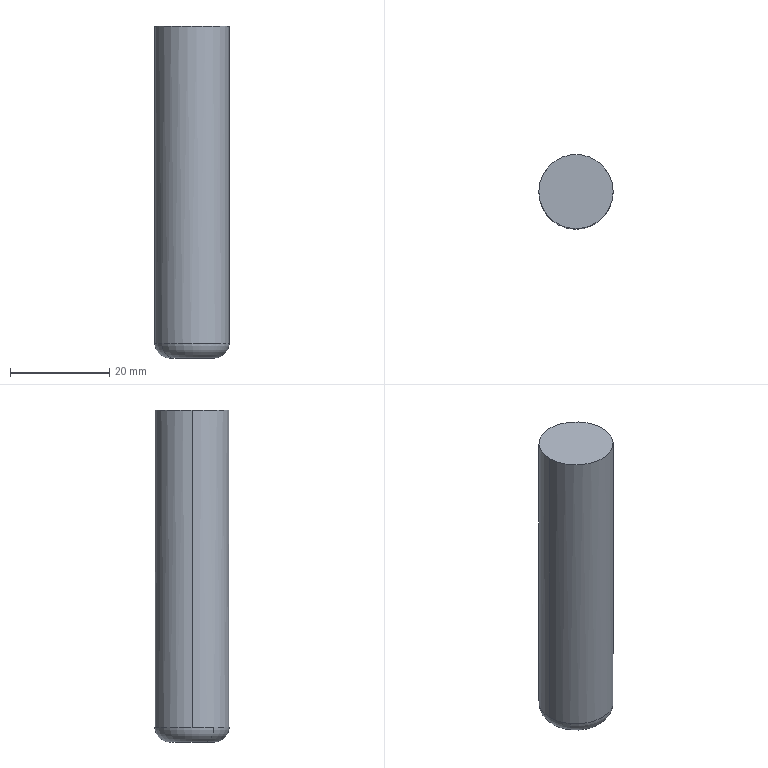Part | 1 solid | 6 faces | box 15 x 15 x 67 mm | volume 11757 mm3 | cylinder 2 | torus 2 | plane 2 | commonest cylinder face diameters 15 x2
STEP:
#1=CARTESIAN_POINT('',(0.,0.,0.));
#2=DIRECTION('',(0.,0.,1.));
#3=DIRECTION('',(1.,0.,0.));
#4=AXIS2_PLACEMENT_3D('',#1,#2,#3);
#5=CARTESIAN_POINT('',(-168.248,494.5,-238.55));
#6=VERTEX_POINT('',#5);
#7=CARTESIAN_POINT('',(-168.248,494.5,-302.55));
#8=VERTEX_POINT('',#7);
#9=CARTESIAN_POINT('',(-168.248,494.5,-238.55));
#10=DIRECTION('',(0.,0.,-1.));
#11=VECTOR('',#10,1.);
#12=LINE('',#9,#11);
#13=CARTESIAN_POINT('',(-160.748,494.5,-238.55));
#14=DIRECTION('',(0.,0.,-1.));
#15=DIRECTION('',(0.,-1.,0.));
#16=AXIS2_PLACEMENT_3D('',#13,#14,#15);
#17=CYLINDRICAL_SURFACE('',#16,7.5);
#18=CARTESIAN_POINT('',(1.571,0.));
#19=DIRECTION('',(0.,1.));
#20=VECTOR('',#19,1.);
#21=LINE('',#18,#20);
#22=(GEOMETRIC_REPRESENTATION_CONTEXT(2)PARAMETRIC_REPRESENTATION_CONTEXT()REPRESENTATION_CONTEXT('',''));
#23=DEFINITIONAL_REPRESENTATION('',(#21),#22);
#24=PCURVE('',#17,#23);
#25=CARTESIAN_POINT('',(-160.748,494.5,-238.55));
#26=DIRECTION('',(0.,0.,-1.));
#27=DIRECTION('',(0.,1.,0.));
#28=AXIS2_PLACEMENT_3D('',#25,#26,#27);
#29=CYLINDRICAL_SURFACE('',#28,7.5);
#30=CARTESIAN_POINT('',(4.712,0.));
#31=DIRECTION('',(0.,1.));
#32=VECTOR('',#31,1.);
#33=LINE('',#30,#32);
#34=(GEOMETRIC_REPRESENTATION_CONTEXT(2)PARAMETRIC_REPRESENTATION_CONTEXT()REPRESENTATION_CONTEXT('',''));
#35=DEFINITIONAL_REPRESENTATION('',(#33),#34);
#36=PCURVE('',#29,#35);
#37=SURFACE_CURVE('',#12,(#24,#36),.PCURVE_S1.);
#38=EDGE_CURVE('',#6,#8,#37,.T.);
#39=ORIENTED_EDGE('',*,*,#38,.F.);
#40=CARTESIAN_POINT('',(-153.248,494.5,-238.55));
#41=VERTEX_POINT('',#40);
#42=CARTESIAN_POINT('',(-160.748,494.5,-238.55));
#43=DIRECTION('',(0.,0.,-1.));
#44=DIRECTION('',(1.,0.,0.));
#45=AXIS2_PLACEMENT_3D('',#42,#43,#44);
#46=CIRCLE('',#45,7.5);
#47=CARTESIAN_POINT('',(-1.571,0.));
#48=DIRECTION('',(1.,0.));
#49=VECTOR('',#48,1.);
#50=LINE('',#47,#49);
#51=(GEOMETRIC_REPRESENTATION_CONTEXT(2)PARAMETRIC_REPRESENTATION_CONTEXT()REPRESENTATION_CONTEXT('',''));
#52=DEFINITIONAL_REPRESENTATION('',(#50),#51);
#53=PCURVE('',#17,#52);
#54=CARTESIAN_POINT('',(-160.748,494.5,-238.55));
#55=DIRECTION('',(0.,0.,-1.));
#56=DIRECTION('',(1.,0.,0.));
#57=AXIS2_PLACEMENT_3D('',#54,#55,#56);
#58=PLANE('',#57);
#59=CARTESIAN_POINT('',(0.,0.));
#60=DIRECTION('',(1.,0.));
#61=AXIS2_PLACEMENT_2D('',#59,#60);
#62=CIRCLE('',#61,7.5);
#63=(GEOMETRIC_REPRESENTATION_CONTEXT(2)PARAMETRIC_REPRESENTATION_CONTEXT()REPRESENTATION_CONTEXT('',''));
#64=DEFINITIONAL_REPRESENTATION('',(#62),#63);
#65=PCURVE('',#58,#64);
#66=SURFACE_CURVE('',#46,(#53,#65),.PCURVE_S1.);
#67=EDGE_CURVE('',#6,#41,#66,.T.);
#68=ORIENTED_EDGE('',*,*,#67,.T.);
#69=CARTESIAN_POINT('',(-153.248,494.5,-302.55));
#70=VERTEX_POINT('',#69);
#71=CARTESIAN_POINT('',(-153.248,494.5,-238.55));
#72=DIRECTION('',(0.,0.,-1.));
#73=VECTOR('',#72,1.);
#74=LINE('',#71,#73);
#75=CARTESIAN_POINT('',(4.712,0.));
#76=DIRECTION('',(0.,1.));
#77=VECTOR('',#76,1.);
#78=LINE('',#75,#77);
#79=(GEOMETRIC_REPRESENTATION_CONTEXT(2)PARAMETRIC_REPRESENTATION_CONTEXT()REPRESENTATION_CONTEXT('',''));
#80=DEFINITIONAL_REPRESENTATION('',(#78),#79);
#81=PCURVE('',#17,#80);
#82=CARTESIAN_POINT('',(1.571,0.));
#83=DIRECTION('',(0.,1.));
#84=VECTOR('',#83,1.);
#85=LINE('',#82,#84);
#86=(GEOMETRIC_REPRESENTATION_CONTEXT(2)PARAMETRIC_REPRESENTATION_CONTEXT()REPRESENTATION_CONTEXT('',''));
#87=DEFINITIONAL_REPRESENTATION('',(#85),#86);
#88=PCURVE('',#29,#87);
#89=SURFACE_CURVE('',#74,(#81,#88),.PCURVE_S1.);
#90=EDGE_CURVE('',#41,#70,#89,.T.);
#91=ORIENTED_EDGE('',*,*,#90,.T.);
#92=CARTESIAN_POINT('',(-154.68,498.909,-302.55));
#93=VERTEX_POINT('',#92);
#94=CARTESIAN_POINT('',(-160.748,494.5,-302.55));
#95=DIRECTION('',(0.,0.,1.));
#96=DIRECTION('',(-0.809,0.5878,0.));
#97=AXIS2_PLACEMENT_3D('',#94,#95,#96);
#98=CIRCLE('',#97,7.5);
#99=CARTESIAN_POINT('',(8.482,64.));
#100=DIRECTION('',(-1.,0.));
#101=VECTOR('',#100,1.);
#102=LINE('',#99,#101);
#103=(GEOMETRIC_REPRESENTATION_CONTEXT(2)PARAMETRIC_REPRESENTATION_CONTEXT()REPRESENTATION_CONTEXT('',''));
#104=DEFINITIONAL_REPRESENTATION('',(#102),#103);
#105=PCURVE('',#17,#104);
#106=CARTESIAN_POINT('',(-160.748,494.5,-302.55));
#107=DIRECTION('',(0.,0.,-1.));
#108=DIRECTION('',(-0.5878,0.809,0.));
#109=AXIS2_PLACEMENT_3D('',#106,#107,#108);
#110=TOROIDAL_SURFACE('',#109,4.5,3.);
#111=CARTESIAN_POINT('',(5.969,0.));
#112=DIRECTION('',(-1.,0.));
#113=VECTOR('',#112,1.);
#114=LINE('',#111,#113);
#115=(GEOMETRIC_REPRESENTATION_CONTEXT(2)PARAMETRIC_REPRESENTATION_CONTEXT()REPRESENTATION_CONTEXT('',''));
#116=DEFINITIONAL_REPRESENTATION('',(#114),#115);
#117=PCURVE('',#110,#116);
#118=SURFACE_CURVE('',#98,(#105,#117),.PCURVE_S1.);
#119=EDGE_CURVE('',#70,#93,#118,.T.);
#120=ORIENTED_EDGE('',*,*,#119,.T.);
#121=CARTESIAN_POINT('',(-166.815,498.909,-302.55));
#122=VERTEX_POINT('',#121);
#123=CARTESIAN_POINT('',(-160.748,494.5,-302.55));
#124=DIRECTION('',(0.,0.,1.));
#125=DIRECTION('',(-0.809,0.5878,0.));
#126=AXIS2_PLACEMENT_3D('',#123,#124,#125);
#127=CIRCLE('',#126,7.5);
#128=CARTESIAN_POINT('',(8.482,64.));
#129=DIRECTION('',(-1.,0.));
#130=VECTOR('',#129,1.);
#131=LINE('',#128,#130);
#132=(GEOMETRIC_REPRESENTATION_CONTEXT(2)PARAMETRIC_REPRESENTATION_CONTEXT()REPRESENTATION_CONTEXT('',''));
#133=DEFINITIONAL_REPRESENTATION('',(#131),#132);
#134=PCURVE('',#17,#133);
#135=CARTESIAN_POINT('',(-160.748,494.5,-302.55));
#136=DIRECTION('',(0.,0.,-1.));
#137=DIRECTION('',(0.5878,-0.809,0.));
#138=AXIS2_PLACEMENT_3D('',#135,#136,#137);
#139=TOROIDAL_SURFACE('',#138,4.5,3.);
#140=CARTESIAN_POINT('',(9.111,0.));
#141=DIRECTION('',(-1.,0.));
#142=VECTOR('',#141,1.);
#143=LINE('',#140,#142);
#144=(GEOMETRIC_REPRESENTATION_CONTEXT(2)PARAMETRIC_REPRESENTATION_CONTEXT()REPRESENTATION_CONTEXT('',''));
#145=DEFINITIONAL_REPRESENTATION('',(#143),#144);
#146=PCURVE('',#139,#145);
#147=SURFACE_CURVE('',#127,(#134,#146),.PCURVE_S1.);
#148=EDGE_CURVE('',#93,#122,#147,.T.);
#149=ORIENTED_EDGE('',*,*,#148,.T.);
#150=CARTESIAN_POINT('',(-160.748,494.5,-302.55));
#151=DIRECTION('',(0.,0.,1.));
#152=DIRECTION('',(-0.809,0.5878,0.));
#153=AXIS2_PLACEMENT_3D('',#150,#151,#152);
#154=CIRCLE('',#153,7.5);
#155=CARTESIAN_POINT('',(2.199,64.));
#156=DIRECTION('',(-1.,0.));
#157=VECTOR('',#156,1.);
#158=LINE('',#155,#157);
#159=(GEOMETRIC_REPRESENTATION_CONTEXT(2)PARAMETRIC_REPRESENTATION_CONTEXT()REPRESENTATION_CONTEXT('',''));
#160=DEFINITIONAL_REPRESENTATION('',(#158),#159);
#161=PCURVE('',#17,#160);
#162=CARTESIAN_POINT('',(2.827,0.));
#163=DIRECTION('',(-1.,0.));
#164=VECTOR('',#163,1.);
#165=LINE('',#162,#164);
#166=(GEOMETRIC_REPRESENTATION_CONTEXT(2)PARAMETRIC_REPRESENTATION_CONTEXT()REPRESENTATION_CONTEXT('',''));
#167=DEFINITIONAL_REPRESENTATION('',(#165),#166);
#168=PCURVE('',#139,#167);
#169=SURFACE_CURVE('',#154,(#161,#168),.PCURVE_S1.);
#170=EDGE_CURVE('',#122,#8,#169,.T.);
#171=ORIENTED_EDGE('',*,*,#170,.T.);
#172=EDGE_LOOP('',(#39,#68,#91,#120,#149,#171));
#173=FACE_BOUND('',#172,.T.);
#174=ADVANCED_FACE('',(#173),#17,.T.);
#175=CARTESIAN_POINT('',(-164.388,491.855,-305.55));
#176=VERTEX_POINT('',#175);
#177=CARTESIAN_POINT('',(-166.815,490.092,-302.55));
#178=VERTEX_POINT('',#177);
#179=CARTESIAN_POINT('',(-164.388,491.855,-302.55));
#180=DIRECTION('',(-0.5878,0.809,0.));
#181=DIRECTION('',(0.,0.,-1.));
#182=AXIS2_PLACEMENT_3D('',#179,#180,#181);
#183=CIRCLE('',#182,3.);
#184=CARTESIAN_POINT('',(1.571,1.571));
#185=DIRECTION('',(0.,-1.));
#186=VECTOR('',#185,1.);
#187=LINE('',#184,#186);
#188=(GEOMETRIC_REPRESENTATION_CONTEXT(2)PARAMETRIC_REPRESENTATION_CONTEXT()REPRESENTATION_CONTEXT('',''));
#189=DEFINITIONAL_REPRESENTATION('',(#187),#188);
#190=PCURVE('',#139,#189);
#191=CARTESIAN_POINT('',(4.712,1.571));
#192=DIRECTION('',(0.,-1.));
#193=VECTOR('',#192,1.);
#194=LINE('',#191,#193);
#195=(GEOMETRIC_REPRESENTATION_CONTEXT(2)PARAMETRIC_REPRESENTATION_CONTEXT()REPRESENTATION_CONTEXT('',''));
#196=DEFINITIONAL_REPRESENTATION('',(#194),#195);
#197=PCURVE('',#110,#196);
#198=SURFACE_CURVE('',#183,(#190,#197),.PCURVE_S1.);
#199=EDGE_CURVE('',#176,#178,#198,.T.);
#200=ORIENTED_EDGE('',*,*,#199,.T.);
#201=CARTESIAN_POINT('',(-160.748,494.5,-302.55));
#202=DIRECTION('',(0.,0.,1.));
#203=DIRECTION('',(-0.809,0.5878,0.));
#204=AXIS2_PLACEMENT_3D('',#201,#202,#203);
#205=CIRCLE('',#204,7.5);
#206=CARTESIAN_POINT('',(2.827,0.));
#207=DIRECTION('',(-1.,0.));
#208=VECTOR('',#207,1.);
#209=LINE('',#206,#208);
#210=(GEOMETRIC_REPRESENTATION_CONTEXT(2)PARAMETRIC_REPRESENTATION_CONTEXT()REPRESENTATION_CONTEXT('',''));
#211=DEFINITIONAL_REPRESENTATION('',(#209),#210);
#212=PCURVE('',#139,#211);
#213=CARTESIAN_POINT('',(5.341,64.));
#214=DIRECTION('',(-1.,0.));
#215=VECTOR('',#214,1.);
#216=LINE('',#213,#215);
#217=(GEOMETRIC_REPRESENTATION_CONTEXT(2)PARAMETRIC_REPRESENTATION_CONTEXT()REPRESENTATION_CONTEXT('',''));
#218=DEFINITIONAL_REPRESENTATION('',(#216),#217);
#219=PCURVE('',#29,#218);
#220=SURFACE_CURVE('',#205,(#212,#219),.PCURVE_S1.);
#221=EDGE_CURVE('',#8,#178,#220,.T.);
#222=ORIENTED_EDGE('',*,*,#221,.F.);
#223=ORIENTED_EDGE('',*,*,#170,.F.);
#224=ORIENTED_EDGE('',*,*,#148,.F.);
#225=CARTESIAN_POINT('',(-157.107,497.145,-305.55));
#226=VERTEX_POINT('',#225);
#227=CARTESIAN_POINT('',(-157.107,497.145,-302.55));
#228=DIRECTION('',(0.5878,-0.809,0.));
#229=DIRECTION('',(0.,0.,-1.));
#230=AXIS2_PLACEMENT_3D('',#227,#228,#229);
#231=CIRCLE('',#230,3.);
#232=CARTESIAN_POINT('',(4.712,1.571));
#233=DIRECTION('',(0.,-1.));
#234=VECTOR('',#233,1.);
#235=LINE('',#232,#234);
#236=(GEOMETRIC_REPRESENTATION_CONTEXT(2)PARAMETRIC_REPRESENTATION_CONTEXT()REPRESENTATION_CONTEXT('',''));
#237=DEFINITIONAL_REPRESENTATION('',(#235),#236);
#238=PCURVE('',#139,#237);
#239=CARTESIAN_POINT('',(1.571,1.571));
#240=DIRECTION('',(0.,-1.));
#241=VECTOR('',#240,1.);
#242=LINE('',#239,#241);
#243=(GEOMETRIC_REPRESENTATION_CONTEXT(2)PARAMETRIC_REPRESENTATION_CONTEXT()REPRESENTATION_CONTEXT('',''));
#244=DEFINITIONAL_REPRESENTATION('',(#242),#243);
#245=PCURVE('',#110,#244);
#246=SURFACE_CURVE('',#231,(#238,#245),.PCURVE_S1.);
#247=EDGE_CURVE('',#226,#93,#246,.T.);
#248=ORIENTED_EDGE('',*,*,#247,.F.);
#249=CARTESIAN_POINT('',(-164.388,497.145,-305.55));
#250=VERTEX_POINT('',#249);
#251=CARTESIAN_POINT('',(-160.748,494.5,-305.55));
#252=DIRECTION('',(0.,0.,-1.));
#253=DIRECTION('',(-0.809,0.5878,0.));
#254=AXIS2_PLACEMENT_3D('',#251,#252,#253);
#255=CIRCLE('',#254,4.5);
#256=CARTESIAN_POINT('',(2.827,1.571));
#257=DIRECTION('',(1.,0.));
#258=VECTOR('',#257,1.);
#259=LINE('',#256,#258);
#260=(GEOMETRIC_REPRESENTATION_CONTEXT(2)PARAMETRIC_REPRESENTATION_CONTEXT()REPRESENTATION_CONTEXT('',''));
#261=DEFINITIONAL_REPRESENTATION('',(#259),#260);
#262=PCURVE('',#139,#261);
#263=CARTESIAN_POINT('',(-160.748,494.5,-305.55));
#264=DIRECTION('',(0.,0.,-1.));
#265=DIRECTION('',(1.,0.,0.));
#266=AXIS2_PLACEMENT_3D('',#263,#264,#265);
#267=PLANE('',#266);
#268=CARTESIAN_POINT('',(0.,0.));
#269=DIRECTION('',(-0.809,-0.5878));
#270=AXIS2_PLACEMENT_2D('',#268,#269);
#271=CIRCLE('',#270,4.5);
#272=(GEOMETRIC_REPRESENTATION_CONTEXT(2)PARAMETRIC_REPRESENTATION_CONTEXT()REPRESENTATION_CONTEXT('',''));
#273=DEFINITIONAL_REPRESENTATION('',(#271),#272);
#274=PCURVE('',#267,#273);
#275=SURFACE_CURVE('',#255,(#262,#274),.PCURVE_S1.);
#276=EDGE_CURVE('',#250,#226,#275,.T.);
#277=ORIENTED_EDGE('',*,*,#276,.F.);
#278=CARTESIAN_POINT('',(-160.748,494.5,-305.55));
#279=DIRECTION('',(0.,0.,-1.));
#280=DIRECTION('',(-0.809,0.5878,0.));
#281=AXIS2_PLACEMENT_3D('',#278,#279,#280);
#282=CIRCLE('',#281,4.5);
#283=CARTESIAN_POINT('',(-3.456,1.571));
#284=DIRECTION('',(1.,0.));
#285=VECTOR('',#284,1.);
#286=LINE('',#283,#285);
#287=(GEOMETRIC_REPRESENTATION_CONTEXT(2)PARAMETRIC_REPRESENTATION_CONTEXT()REPRESENTATION_CONTEXT('',''));
#288=DEFINITIONAL_REPRESENTATION('',(#286),#287);
#289=PCURVE('',#139,#288);
#290=CARTESIAN_POINT('',(0.,0.));
#291=DIRECTION('',(-0.809,-0.5878));
#292=AXIS2_PLACEMENT_2D('',#290,#291);
#293=CIRCLE('',#292,4.5);
#294=(GEOMETRIC_REPRESENTATION_CONTEXT(2)PARAMETRIC_REPRESENTATION_CONTEXT()REPRESENTATION_CONTEXT('',''));
#295=DEFINITIONAL_REPRESENTATION('',(#293),#294);
#296=PCURVE('',#267,#295);
#297=SURFACE_CURVE('',#282,(#289,#296),.PCURVE_S1.);
#298=EDGE_CURVE('',#176,#250,#297,.T.);
#299=ORIENTED_EDGE('',*,*,#298,.F.);
#300=EDGE_LOOP('',(#200,#222,#223,#224,#248,#277,#299));
#301=FACE_BOUND('',#300,.T.);
#302=ADVANCED_FACE('',(#301),#139,.T.);
#303=ORIENTED_EDGE('',*,*,#276,.T.);
#304=CARTESIAN_POINT('',(-160.748,494.5,-305.55));
#305=DIRECTION('',(0.,0.,-1.));
#306=DIRECTION('',(-0.809,0.5878,0.));
#307=AXIS2_PLACEMENT_3D('',#304,#305,#306);
#308=CIRCLE('',#307,4.5);
#309=CARTESIAN_POINT('',(0.,0.));
#310=DIRECTION('',(-0.809,-0.5878));
#311=AXIS2_PLACEMENT_2D('',#309,#310);
#312=CIRCLE('',#311,4.5);
#313=(GEOMETRIC_REPRESENTATION_CONTEXT(2)PARAMETRIC_REPRESENTATION_CONTEXT()REPRESENTATION_CONTEXT('',''));
#314=DEFINITIONAL_REPRESENTATION('',(#312),#313);
#315=PCURVE('',#267,#314);
#316=CARTESIAN_POINT('',(-0.3142,1.571));
#317=DIRECTION('',(1.,0.));
#318=VECTOR('',#317,1.);
#319=LINE('',#316,#318);
#320=(GEOMETRIC_REPRESENTATION_CONTEXT(2)PARAMETRIC_REPRESENTATION_CONTEXT()REPRESENTATION_CONTEXT('',''));
#321=DEFINITIONAL_REPRESENTATION('',(#319),#320);
#322=PCURVE('',#110,#321);
#323=SURFACE_CURVE('',#308,(#315,#322),.PCURVE_S1.);
#324=EDGE_CURVE('',#226,#176,#323,.T.);
#325=ORIENTED_EDGE('',*,*,#324,.T.);
#326=ORIENTED_EDGE('',*,*,#298,.T.);
#327=EDGE_LOOP('',(#303,#325,#326));
#328=FACE_BOUND('',#327,.T.);
#329=ADVANCED_FACE('',(#328),#267,.T.);
#330=ORIENTED_EDGE('',*,*,#67,.F.);
#331=CARTESIAN_POINT('',(-160.748,494.5,-238.55));
#332=DIRECTION('',(0.,0.,-1.));
#333=DIRECTION('',(1.,0.,0.));
#334=AXIS2_PLACEMENT_3D('',#331,#332,#333);
#335=CIRCLE('',#334,7.5);
#336=CARTESIAN_POINT('',(0.,0.));
#337=DIRECTION('',(1.,0.));
#338=AXIS2_PLACEMENT_2D('',#336,#337);
#339=CIRCLE('',#338,7.5);
#340=(GEOMETRIC_REPRESENTATION_CONTEXT(2)PARAMETRIC_REPRESENTATION_CONTEXT()REPRESENTATION_CONTEXT('',''));
#341=DEFINITIONAL_REPRESENTATION('',(#339),#340);
#342=PCURVE('',#58,#341);
#343=CARTESIAN_POINT('',(1.571,0.));
#344=DIRECTION('',(1.,0.));
#345=VECTOR('',#344,1.);
#346=LINE('',#343,#345);
#347=(GEOMETRIC_REPRESENTATION_CONTEXT(2)PARAMETRIC_REPRESENTATION_CONTEXT()REPRESENTATION_CONTEXT('',''));
#348=DEFINITIONAL_REPRESENTATION('',(#346),#347);
#349=PCURVE('',#29,#348);
#350=SURFACE_CURVE('',#335,(#342,#349),.PCURVE_S1.);
#351=EDGE_CURVE('',#41,#6,#350,.T.);
#352=ORIENTED_EDGE('',*,*,#351,.F.);
#353=EDGE_LOOP('',(#330,#352));
#354=FACE_BOUND('',#353,.T.);
#355=ADVANCED_FACE('',(#354),#58,.F.);
#356=ORIENTED_EDGE('',*,*,#38,.T.);
#357=ORIENTED_EDGE('',*,*,#221,.T.);
#358=CARTESIAN_POINT('',(-160.748,494.5,-302.55));
#359=DIRECTION('',(0.,0.,1.));
#360=DIRECTION('',(-0.809,0.5878,0.));
#361=AXIS2_PLACEMENT_3D('',#358,#359,#360);
#362=CIRCLE('',#361,7.5);
#363=CARTESIAN_POINT('',(5.341,64.));
#364=DIRECTION('',(-1.,0.));
#365=VECTOR('',#364,1.);
#366=LINE('',#363,#365);
#367=(GEOMETRIC_REPRESENTATION_CONTEXT(2)PARAMETRIC_REPRESENTATION_CONTEXT()REPRESENTATION_CONTEXT('',''));
#368=DEFINITIONAL_REPRESENTATION('',(#366),#367);
#369=PCURVE('',#29,#368);
#370=CARTESIAN_POINT('',(5.969,0.));
#371=DIRECTION('',(-1.,0.));
#372=VECTOR('',#371,1.);
#373=LINE('',#370,#372);
#374=(GEOMETRIC_REPRESENTATION_CONTEXT(2)PARAMETRIC_REPRESENTATION_CONTEXT()REPRESENTATION_CONTEXT('',''));
#375=DEFINITIONAL_REPRESENTATION('',(#373),#374);
#376=PCURVE('',#110,#375);
#377=SURFACE_CURVE('',#362,(#369,#376),.PCURVE_S1.);
#378=EDGE_CURVE('',#178,#70,#377,.T.);
#379=ORIENTED_EDGE('',*,*,#378,.T.);
#380=ORIENTED_EDGE('',*,*,#90,.F.);
#381=ORIENTED_EDGE('',*,*,#351,.T.);
#382=EDGE_LOOP('',(#356,#357,#379,#380,#381));
#383=FACE_BOUND('',#382,.T.);
#384=ADVANCED_FACE('',(#383),#29,.T.);
#385=ORIENTED_EDGE('',*,*,#199,.F.);
#386=ORIENTED_EDGE('',*,*,#324,.F.);
#387=ORIENTED_EDGE('',*,*,#247,.T.);
#388=ORIENTED_EDGE('',*,*,#119,.F.);
#389=ORIENTED_EDGE('',*,*,#378,.F.);
#390=EDGE_LOOP('',(#385,#386,#387,#388,#389));
#391=FACE_BOUND('',#390,.T.);
#392=ADVANCED_FACE('',(#391),#110,.T.);
#393=CLOSED_SHELL('',(#174,#302,#329,#355,#384,#392));
#394=MANIFOLD_SOLID_BREP('',#393);
#395=(LENGTH_UNIT()NAMED_UNIT(*)SI_UNIT(.MILLI.,.METRE.));
#396=UNCERTAINTY_MEASURE_WITH_UNIT(LENGTH_MEASURE(0.0000001),#395,'','');
#397=(NAMED_UNIT(*)PLANE_ANGLE_UNIT()SI_UNIT($,.RADIAN.));
#398=(NAMED_UNIT(*)SI_UNIT($,.STERADIAN.)SOLID_ANGLE_UNIT());
#399=(GEOMETRIC_REPRESENTATION_CONTEXT(3)GLOBAL_UNCERTAINTY_ASSIGNED_CONTEXT((#396))GLOBAL_UNIT_ASSIGNED_CONTEXT((#395,#397,#398))REPRESENTATION_CONTEXT('',''));
#400=ADVANCED_BREP_SHAPE_REPRESENTATION('',(#4,#394),#399);